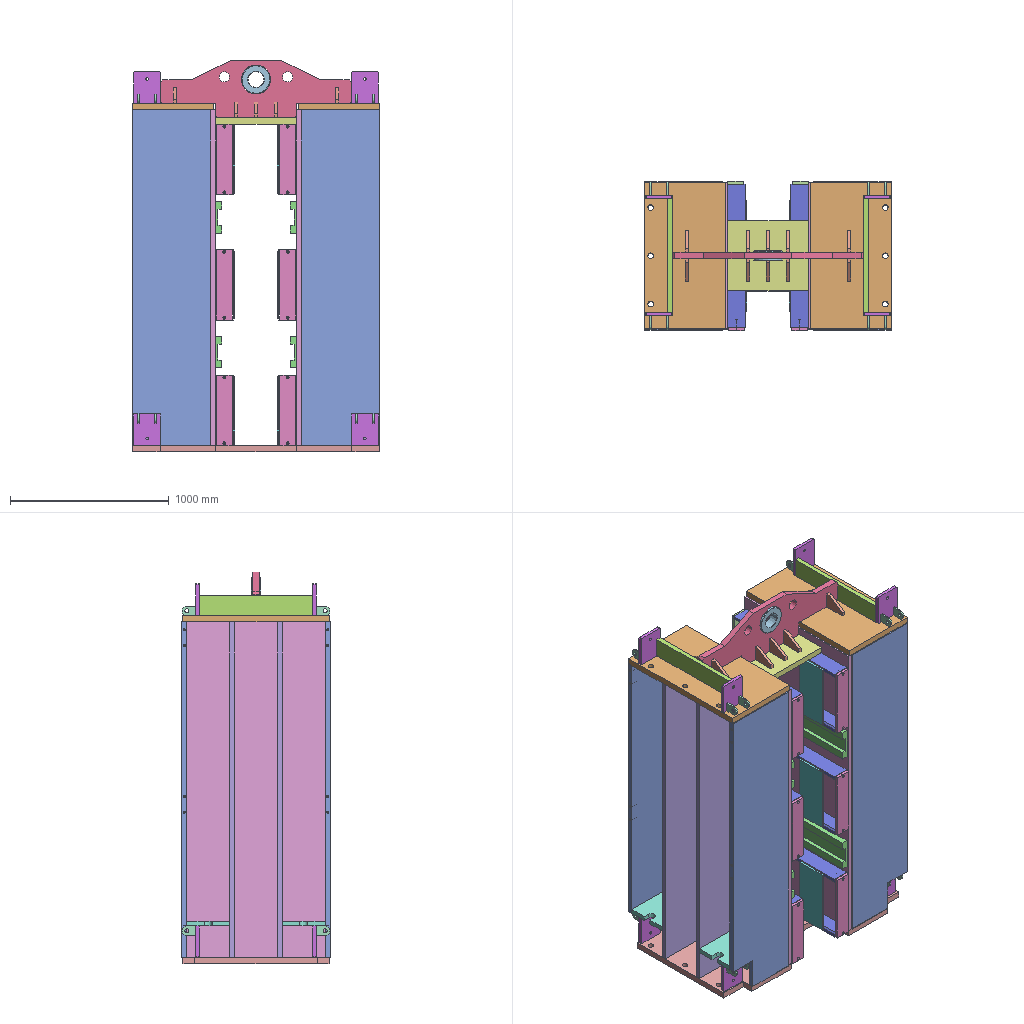Assembly | SolidWorks | 20 different items | 110 placed | box 1560 x 940 x 2473 mm
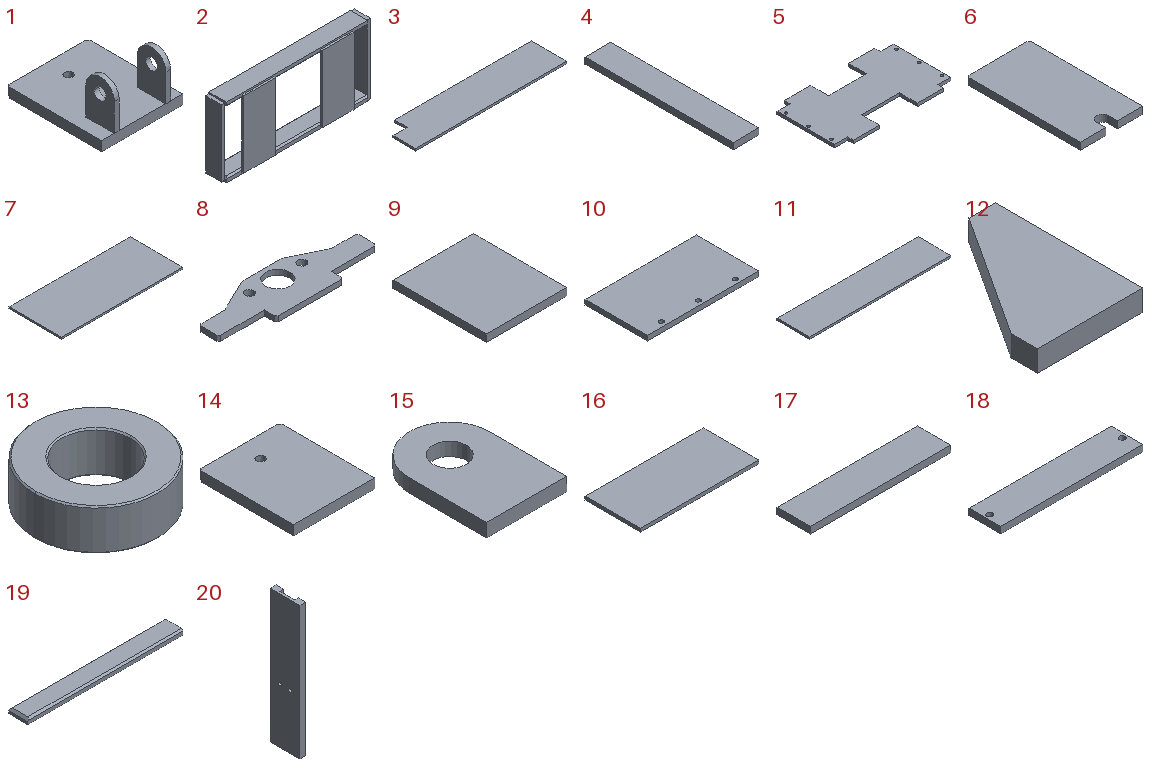Parts list (item | name | quantity | parent item | size | volume | features):
1 | (subassembly) | x8 | - | 170 x 200 x 108 mm | 763193 mm3 | -
2 | (subassembly) | x6 | - | 940 x 122 x 445 mm | 9500591 mm3 | -
3 | - | x4 | - | 2118 x 492 x 30 mm | 30183108 mm3 | features 3DProfileFeature 1, Extrusion 1, HoleWzd 1
4 | - | x2 | - | 125 x 718 x 30 mm | 2692500 mm3 | features Extrusion 1
5 | - | x1 | - | 1560 x 922 x 40 mm | 45355710 mm3 | features Extrusion 1
6 | - | x4 | - | 270 x 492 x 30 mm | 3892748 mm3 | features Extrusion 1
7 | - | x2 | - | 2118 x 922 x 30 mm | 58583880 mm3 | features Extrusion 1
8 | - | x1 | - | 1205 x 365 x 40 mm | 10483325 mm3 | features Extrusion 1
9 | - | x1 | - | 440 x 510 x 40 mm | 8976000 mm3 | features Extrusion 1
10 | - | x2 | - | 922 x 515 x 40 mm | 18871055 mm3 | features Extrusion 1
11 | - | x4 | - | 2118 x 492 x 30 mm | 31261680 mm3 | features Extrusion 1
12 | - | x10 | - | 100 x 140 x 20 mm | 193750 mm3 | features Extrusion 1
13 | - | x1 | - | 180 x 180 x 60 mm | 1052057 mm3 | features Chamfer 1, Extrusion 1
14 | - | x8 | in 1 | 170 x 200 x 20 mm | 675136 mm3 | features 3DProfileFeature 1, Extrusion 1, HoleWzd 1
15 | - | x16 | in 1 | 60 x 88 x 10 mm | 44028 mm3 | features Extrusion 1
16 | - | x12 | in 2 | 425 x 200 x 12 mm | 1020000 mm3 | features Extrusion 1
17 | - | x6 | in 2 | 425 x 100 x 20 mm | 850000 mm3 | features Extrusion 1
18 | - | x6 | in 2 | 445 x 100 x 20 mm | 879821 mm3 | features Extrusion 1
19 | - | x12 | in 2 | 900 x 110 x 30 mm | 2865385 mm3 | features Chamfer 2, 3DProfileFeature 1, Extrusion 1, HoleWzd 1
20 | - | x4 | - | 40 x 200 x 900 mm | 4927112 mm3 | features 3DProfileFeature 1, Extrusion 1, HoleWzd 1
Mates (type | each side: item.copy, entity, surface, feature):
In the top assembly
Coincident | 5.1 face plane Boss-Extrude1 | 7.1 face plane Boss-Extrude1 | 2 times
Coincident | 5.1 face plane Boss-Extrude1 | 7.2 face plane Boss-Extrude1 | 2 times
DistanceDim | 7.1 face plane Boss-Extrude1 | 7.2 face plane Boss-Extrude1
Coincident | 7.2 face plane Boss-Extrude1 | 7.1 face plane Boss-Extrude1
Coincident | 7.1 face plane Boss-Extrude1 | 6.1 face plane Boss-Extrude1
Coincident | 6.1 face plane Boss-Extrude1 | 6.2 face plane Boss-Extrude1 | 2 times
Coincident | 6.3 face plane Boss-Extrude1 | 6.4 face plane Boss-Extrude1 | 2 times
Coincident | 7.2 face plane Boss-Extrude1 | 6.3 face plane Boss-Extrude1
Coincident | 6.4 face plane Boss-Extrude1 | 6.1 face plane Boss-Extrude1
Coincident | 7.1 face plane Boss-Extrude1 | 10.1 face plane Boss-Extrude1 | 2 times
Coincident | 10.2 face plane Boss-Extrude1 | 10.1 face plane Boss-Extrude1 | 2 times
Coincident | 5.1 face plane Boss-Extrude1 | 11.1 face plane Boss-Extrude1
Coincident | 7.1 face plane Boss-Extrude1 | 11.1 face plane Boss-Extrude1
Coincident | 5.1 face plane Boss-Extrude1 | 11.2 face plane Boss-Extrude1
Coincident | 7.2 face plane Boss-Extrude1 | 11.2 face plane Boss-Extrude1
Coincident | 11.1 face plane Boss-Extrude1 | 11.2 face plane Boss-Extrude1
Coincident | 5.1 face plane Boss-Extrude1 | 11.3 face plane Boss-Extrude1
Coincident | 7.1 face plane Boss-Extrude1 | 11.3 face plane Boss-Extrude1
Coincident | 7.2 face plane Boss-Extrude1 | 11.4 face plane Boss-Extrude1
Coincident | 11.3 face plane Boss-Extrude1 | 11.4 face plane Boss-Extrude1
DistanceDim | 11.4 face plane Boss-Extrude1 | 11.2 face plane Boss-Extrude1
Coincident | 6.1 face plane Boss-Extrude1 | 11.3 face plane Boss-Extrude1
Coincident | 6.2 face plane Boss-Extrude1 | 11.1 face plane Boss-Extrude1
Coincident | 6.3 face plane Boss-Extrude1 | 6.1 face plane Boss-Extrude1
Coincident | 6.4 face plane Boss-Extrude1 | 6.2 face plane Boss-Extrude1
Coincident | 5.1 face plane Boss-Extrude1 | 11.4 face plane Boss-Extrude1
DistanceDim | 11.4 face plane Boss-Extrude1 | 5.1 face plane Boss-Extrude1
Coincident | 3.1 face plane Boss-Extrude1 | 7.2 face plane Boss-Extrude1
Coincident | 3.2 face plane Boss-Extrude1 | 7.2 face plane Boss-Extrude1
DistanceDim | 3.1 face plane Boss-Extrude1 | 3.2 face plane Boss-Extrude1
Coincident | 5.1 face plane Boss-Extrude1 | 3.1 face plane Boss-Extrude1
DistanceDim | 3.1 face plane Boss-Extrude1 | 5.1 face plane Boss-Extrude1
Coincident | 5.1 face plane Boss-Extrude1 | 3.2 face plane Boss-Extrude1
Coincident | 3.3 face plane Boss-Extrude1 | 5.1 face plane Boss-Extrude1
Coincident | 3.3 face plane Boss-Extrude1 | 7.1 face plane Boss-Extrude1
Coincident | 3.3 face plane Boss-Extrude1 | 3.1 face plane Boss-Extrude1
Coincident | 5.1 face plane Boss-Extrude1 | 3.4 face plane Boss-Extrude1
Coincident | 3.4 face plane Boss-Extrude1 | 3.2 face plane Boss-Extrude1
Coincident | 3.4 face plane Boss-Extrude1 | 7.1 face plane Boss-Extrude1
Coincident | 3.3 face plane Boss-Extrude1 | 6.2 face plane Boss-Extrude1
Coincident | 7.1 face plane Boss-Extrude1 | 20.1 face plane Boss-Extrude1
Coincident | 20.1 face plane Boss-Extrude1 | 20.2 face plane Boss-Extrude1 | 2 times
Coincident | 7.2 face plane Boss-Extrude1 | 20.3 face plane Boss-Extrude1
Coincident | 7.2 face plane Boss-Extrude1 | 20.4 face plane Boss-Extrude1
DistanceDim | 20.4 face plane Boss-Extrude1 | 20.3 face plane Boss-Extrude1
Coincident | 20.3 face plane Boss-Extrude1 | 20.4 face plane Boss-Extrude1
DistanceDim | 20.1 face plane Boss-Extrude1 | 20.2 face plane Boss-Extrude1
Coincident | 20.2 face plane Boss-Extrude1 | 20.4 face plane Boss-Extrude1
DistanceDim | 20.2 face plane Boss-Extrude1 | 7.1 face plane Boss-Extrude1
DistanceDim | 20.3 face plane Boss-Extrude1 | 5.1 face plane Boss-Extrude1
Coincident | 20.1 face plane Boss-Extrude1 | 20.3 face plane Boss-Extrude1
Concentric | 8.1 face cylinder Boss-Extrude1 | 13.1 face cylinder Boss-Extrude1
DistanceDim | 13.1 face plane Boss-Extrude1 | 8.1 face plane Boss-Extrude1
Coincident | 10.1 face plane Boss-Extrude1 | 8.1 face plane Boss-Extrude1
Coincident | 8.1 face plane Boss-Extrude1 | 9.1 face plane Boss-Extrude1
Coincident | 7.2 face plane Boss-Extrude1 | 8.1 face plane Boss-Extrude1
Coincident | 7.1 face plane Boss-Extrude1 | 9.1 face plane Boss-Extrude1
DistanceDim | 9.1 face plane Boss-Extrude1 | 7.2 face plane Boss-Extrude1
DistanceDim | 8.1 face plane Boss-Extrude1 | 9.1 face plane Boss-Extrude1
Coincident | 10.1 face plane Boss-Extrude1 | 4.1 face plane Boss-Extrude1
Coincident | 4.2 face plane Boss-Extrude1 | 4.1 face plane Boss-Extrude1 | 2 times
Coincident | 4.1 face plane Boss-Extrude1 | 8.1 face plane Boss-Extrude1
Coincident | 4.2 face plane Boss-Extrude1 | 8.1 face plane Boss-Extrude1
DistanceDim | 4.2 face plane Boss-Extrude1 | 10.1 face plane Boss-Extrude1
Coincident | 14.1 face plane Boss-Extrude1 | 14.2 face plane Boss-Extrude1 | 2 times
Coincident | 14.1 face plane Boss-Extrude1 | 14.3 face plane Boss-Extrude1
Coincident | 14.3 face plane Boss-Extrude1 | 14.4 face plane Boss-Extrude1 | 2 times
Coincident | 10.1 face plane Boss-Extrude1 | 14.2 face plane Boss-Extrude1
Coincident | 4.2 face plane Boss-Extrude1 | 14.4 face plane Boss-Extrude1 | 2 times
Coincident | 14.1 face plane Boss-Extrude1 | 14.4 face plane Boss-Extrude1
Coincident | 4.1 face plane Boss-Extrude1 | 14.1 face plane Boss-Extrude1
Coincident | 14.2 face plane Boss-Extrude1 | 14.3 face plane Boss-Extrude1
Coincident | 4.2 face plane Boss-Extrude1 | 14.3 face plane Boss-Extrude1
Coincident | 5.1 face plane Boss-Extrude1 | 14.5 face plane Boss-Extrude1
Coincident | 14.3 face plane Boss-Extrude1 | 14.5 face plane Boss-Extrude1 | 2 times
Coincident | 5.1 face plane Boss-Extrude1 | 14.6 face plane Boss-Extrude1
Coincident | 14.1 face plane Boss-Extrude1 | 14.6 face plane Boss-Extrude1 | 2 times
Coincident | 5.1 face plane Boss-Extrude1 | 14.7 face plane Boss-Extrude1
Coincident | 14.2 face plane Boss-Extrude1 | 14.7 face plane Boss-Extrude1 | 2 times
Coincident | 5.1 face plane Boss-Extrude1 | 14.8 face plane Boss-Extrude1
Coincident | 14.4 face plane Boss-Extrude1 | 14.8 face plane Boss-Extrude1 | 2 times
Coincident | 5.1 face plane Boss-Extrude1 | 10.2 face plane Boss-Extrude1
Coincident | 5.1 face plane Boss-Extrude1 | 10.1 face plane Boss-Extrude1
Coincident | 10.1 face plane Boss-Extrude1 | 12.1 face plane Boss-Extrude1
Coincident | 12.1 face plane Boss-Extrude1 | 12.2 face plane Boss-Extrude1 | 2 times
Coincident | 8.1 face plane Boss-Extrude1 | 12.1 face plane Boss-Extrude1
Coincident | 12.2 face plane Boss-Extrude1 | 12.3 face plane Boss-Extrude1
Coincident | 12.2 face plane Boss-Extrude1 | 12.4 face plane Boss-Extrude1
Coincident | 12.2 face plane Boss-Extrude1 | 12.5 face plane Boss-Extrude1
Coincident | 9.1 face plane Boss-Extrude1 | 12.3 face plane Boss-Extrude1
Coincident | 12.5 face plane Boss-Extrude1 | 12.3 face plane Boss-Extrude1
Coincident | 12.3 face plane Boss-Extrude1 | 12.4 face plane Boss-Extrude1
Coincident | 12.6 face plane Boss-Extrude1 | 12.4 face plane Boss-Extrude1 | 2 times
Coincident | 8.1 face plane Boss-Extrude1 | 12.6 face plane Boss-Extrude1
Coincident | 12.7 face plane Boss-Extrude1 | 12.6 face plane Boss-Extrude1
Coincident | 12.6 face plane Boss-Extrude1 | 12.8 face plane Boss-Extrude1 | 2 times
Coincident | 12.7 face plane Boss-Extrude1 | 12.8 face plane Boss-Extrude1
Coincident | 12.9 face plane Boss-Extrude1 | 12.10 face plane Boss-Extrude1 | 2 times
Coincident | 12.2 face plane Boss-Extrude1 | 12.9 face plane Boss-Extrude1 | 2 times
Coincident | 12.6 face plane Boss-Extrude1 | 12.9 face plane Boss-Extrude1
Coincident | 12.1 face plane Boss-Extrude1 | 12.10 face plane Boss-Extrude1
Coincident | 12.8 face plane Boss-Extrude1 | 12.5 face plane Boss-Extrude1
Coincident | 12.7 face plane Boss-Extrude1 | 12.3 face plane Boss-Extrude1
DistanceDim | 12.6 face plane Boss-Extrude1 | 12.8 face plane Boss-Extrude1
DistanceDim | 13.1 face cylinder Boss-Extrude1 | 12.8 face plane Boss-Extrude1
DistanceDim | 12.7 face plane Boss-Extrude1 | 13.1 face cylinder Boss-Extrude1
DistanceDim | 12.9 face plane Boss-Extrude1 | 12.10 face plane Boss-Extrude1
DistanceDim | 13.1 face cylinder Boss-Extrude1 | 12.9 face plane Boss-Extrude1
Coincident | 7.2 face plane Boss-Extrude1 | 17.1 face plane Boss-Extrude1
Coincident | 9.1 face plane Boss-Extrude1 | 19.1 face plane Boss-Extrude1
DistanceDim | 19.2 face plane Boss-Extrude1 | 7.2 face plane Boss-Extrude1
Coincident | 7.1 face plane Boss-Extrude1 | 19.3 face plane Boss-Extrude1
Coincident | 9.1 face plane Boss-Extrude1 | 19.3 face plane Boss-Extrude1
Coincident | 18.1 face plane Boss-Extrude1 | 18.2 face plane Boss-Extrude1
Coincident | 7.2 face plane Boss-Extrude1 | 19.4 face plane Boss-Extrude1
Coincident | 18.1 face plane Boss-Extrude1 | 18.3 face plane Boss-Extrude1
Coincident | 7.2 face plane Boss-Extrude1 | 19.5 face plane Boss-Extrude1
Coincident | 5.1 face plane Boss-Extrude1 | 19.6 face plane Boss-Extrude1
Coincident | 18.3 face plane Boss-Extrude1 | 18.4 face plane Boss-Extrude1
Coincident | 7.1 face plane Boss-Extrude1 | 19.7 face plane Boss-Extrude1
Coincident | 18.2 face plane Boss-Extrude1 | 18.5 face plane Boss-Extrude1
Coincident | 5.1 face plane Boss-Extrude1 | 19.7 face plane Boss-Extrude1
Coincident | 7.1 face plane Boss-Extrude1 | 19.8 face plane Boss-Extrude1
Coincident | 18.2 face plane Boss-Extrude1 | 18.6 face plane Boss-Extrude1
Coincident | 19.4 face plane Boss-Extrude1 | 19.9 face plane Boss-Extrude1
DistanceDim | 19.4 face plane Boss-Extrude1 | 20.4 face plane Boss-Extrude1
In subassembly 1
Coincident | 14.9 face plane Boss-Extrude1 | 15.1 face plane Boss-Extrude1 | 2 times
Coincident | 14.9 face plane Boss-Extrude1 | 15.2 face plane Boss-Extrude1 | 2 times
DistanceDim | 15.2 face plane Boss-Extrude1 | 15.1 face plane Boss-Extrude1
DistanceDim | 15.1 face plane Boss-Extrude1 | 14.9 face plane Boss-Extrude1
In subassembly 2
Coincident | 19.10 face plane Boss-Extrude1 | 19.11 face plane Boss-Extrude1 | 2 times
Concentric | 19.11 face cylinder M16 Tapped Hole1 | 18.7 face cylinder Boss-Extrude1
Coincident | 19.11 face plane Boss-Extrude1 | 18.7 face plane Boss-Extrude1
Concentric | 19.10 face cylinder M16 Tapped Hole1 | 18.7 face cylinder Boss-Extrude1
Coincident | 19.11 face plane Boss-Extrude1 | 17.2 face plane Boss-Extrude1 | 2 times
DistanceDim | 19.11 face plane Boss-Extrude1 | 17.2 face plane Boss-Extrude1
Coincident | 19.11 face plane Boss-Extrude1 | 16.1 face plane Boss-Extrude1
Coincident | 16.1 face plane Boss-Extrude1 | 16.2 face plane Boss-Extrude1 | 2 times
DistanceDim | 16.1 face plane Boss-Extrude1 | 19.10 face plane Boss-Extrude1
DistanceDim | 16.1 face plane Boss-Extrude1 | 18.7 face plane Boss-Extrude1
DistanceDim | 16.2 face plane Boss-Extrude1 | 17.2 face plane Boss-Extrude1